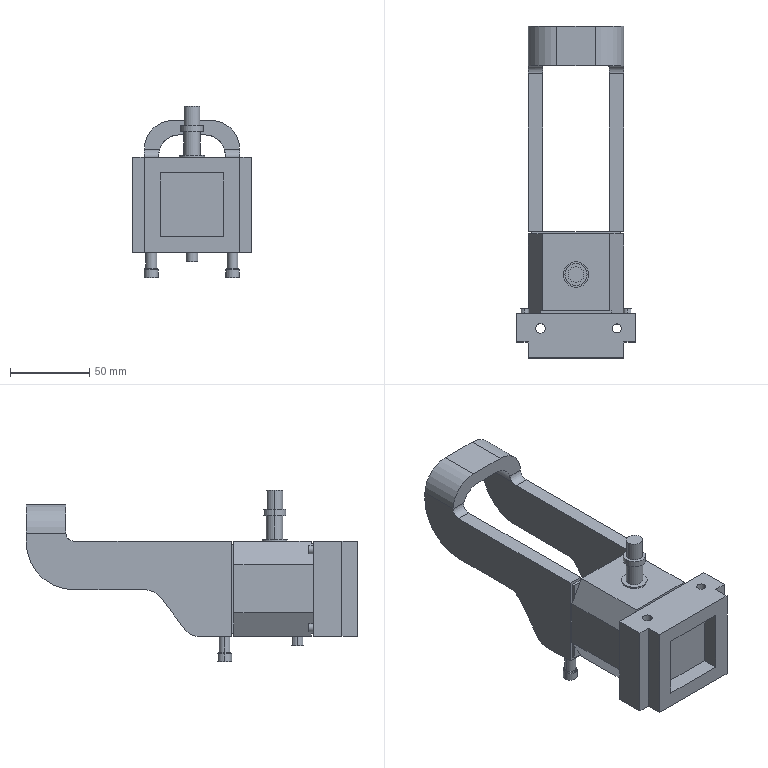Part | SolidWorks | features ICE 21, Fillet 6, MirrorPattern 3, Chamfer 2, Extrusion 1 | 1 solid | 182 faces | box 75 x 208.792 x 108 mm | volume 304724 mm3 | plane 132 | cylinder 50 | commonest cylinder face diameters 5.095 x8 26 x4 5.711 x2 6.154 x2 6.666 x2 6.867 x2